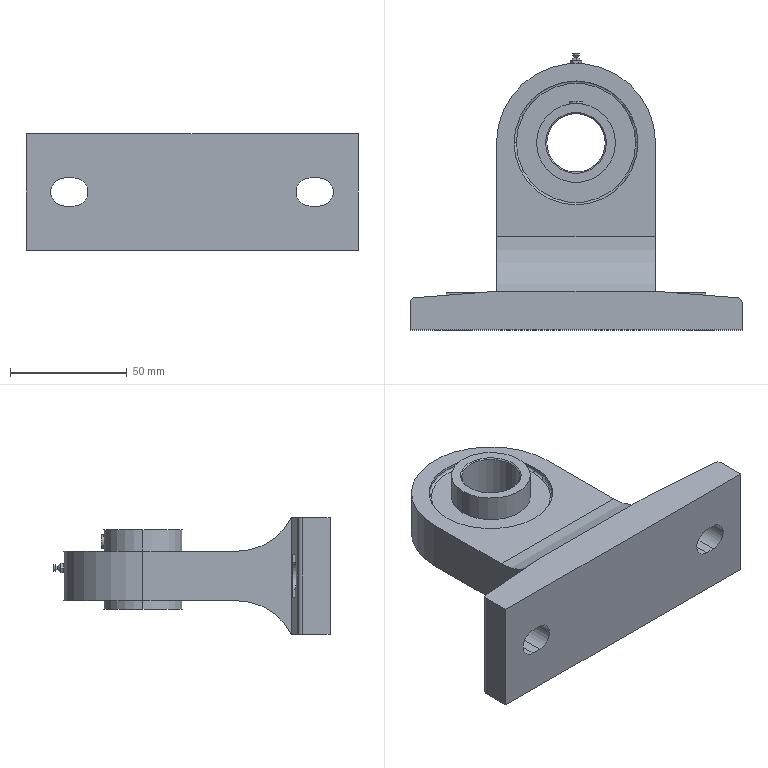Part | SolidWorks | features ICE 3, Revolution 3, Fillet 2, BaseBody 1, Chamfer 1, HoleWzd 1 | 1 solid | 78 faces | box 142 x 118.08 x 50 mm | volume 239637 mm3 | plane 37 | cylinder 23 | cone 14 | torus 4 | commonest cylinder face diameters 12 x4 33.75 x4 53 x4 2.72 x2 4 x2 6 x2